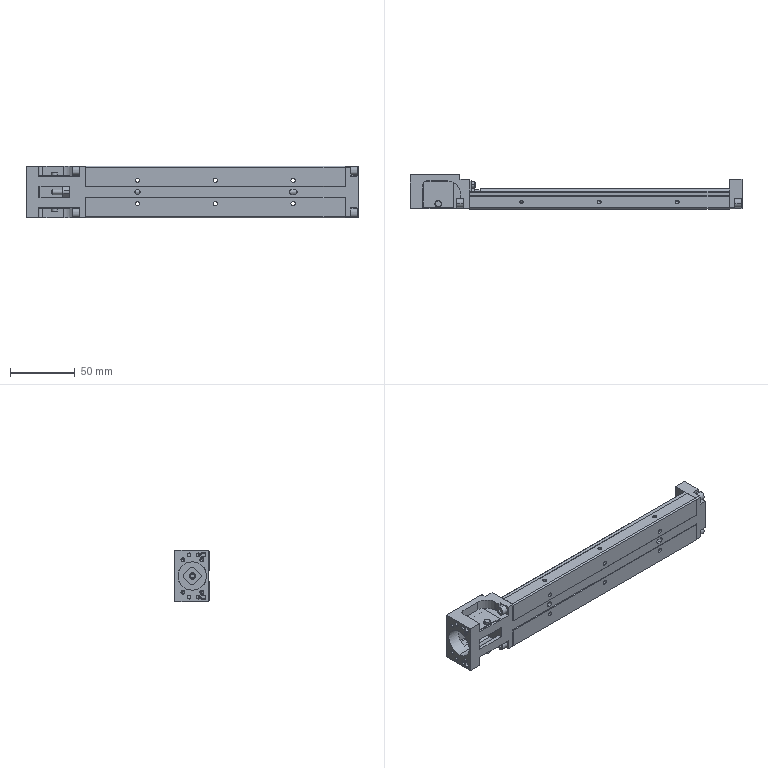Part | STEP file | QA-LX2005C_B1_A2038_200_EP3_b | 1 solid | 346 faces | box 256 x 26.5 x 40 mm | volume 92553 mm3 | plane 175 | cylinder 117 | cone 54 | commonest cylinder face diameters 2.459 x20 4 x14 3.4 x12 4.5 x12 6.5 x12 2.9 x8